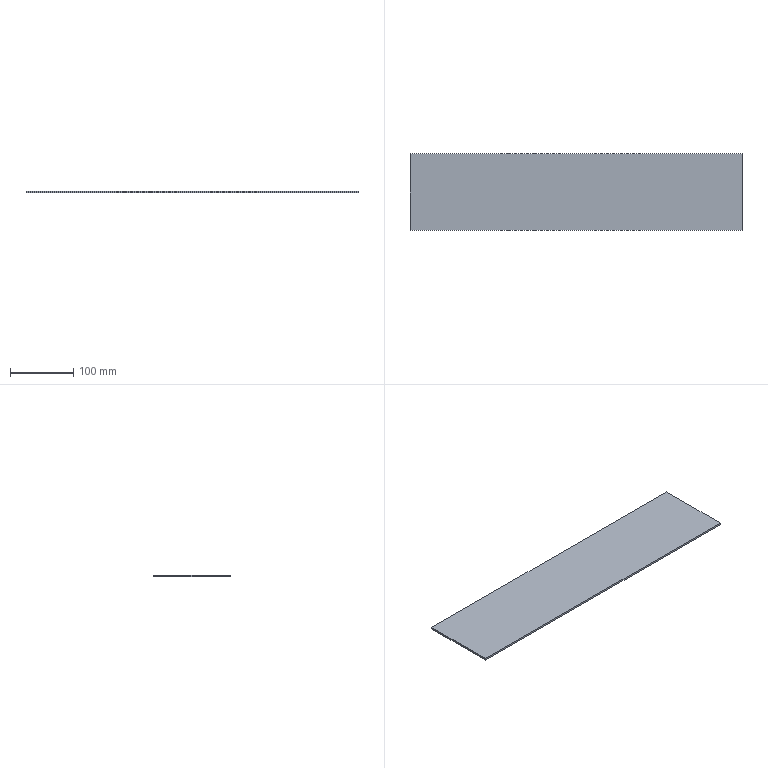Part | STEP file | Double-tube frame vertical brace plate SGN-1-06 | 1 solid | 6 faces | box 523 x 120 x 3 mm | volume 188280 mm3 | plane 6
STEP:
#1=CARTESIAN_POINT('',(0.,0.,0.));
#2=DIRECTION('',(0.,0.,1.));
#3=DIRECTION('',(1.,0.,0.));
#4=AXIS2_PLACEMENT_3D('',#1,#2,#3);
#5=CARTESIAN_POINT('',(261.5,-60.,0.));
#6=VERTEX_POINT('',#5);
#7=CARTESIAN_POINT('',(261.5,60.,0.));
#8=VERTEX_POINT('',#7);
#9=CARTESIAN_POINT('',(261.5,-60.,0.));
#10=DIRECTION('',(0.,1.,0.));
#11=VECTOR('',#10,1.);
#12=LINE('',#9,#11);
#13=CARTESIAN_POINT('',(261.5,-60.,-3.));
#14=DIRECTION('',(1.,0.,0.));
#15=DIRECTION('',(0.,0.,-1.));
#16=AXIS2_PLACEMENT_3D('',#13,#14,#15);
#17=PLANE('',#16);
#18=CARTESIAN_POINT('',(-3.,0.));
#19=DIRECTION('',(0.,1.));
#20=VECTOR('',#19,1.);
#21=LINE('',#18,#20);
#22=(GEOMETRIC_REPRESENTATION_CONTEXT(2)PARAMETRIC_REPRESENTATION_CONTEXT()REPRESENTATION_CONTEXT('',''));
#23=DEFINITIONAL_REPRESENTATION('',(#21),#22);
#24=PCURVE('',#17,#23);
#25=CARTESIAN_POINT('',(0.,0.,0.));
#26=DIRECTION('',(0.,0.,-1.));
#27=DIRECTION('',(-1.,0.,0.));
#28=AXIS2_PLACEMENT_3D('',#25,#26,#27);
#29=PLANE('',#28);
#30=CARTESIAN_POINT('',(-261.5,-60.));
#31=DIRECTION('',(0.,1.));
#32=VECTOR('',#31,1.);
#33=LINE('',#30,#32);
#34=(GEOMETRIC_REPRESENTATION_CONTEXT(2)PARAMETRIC_REPRESENTATION_CONTEXT()REPRESENTATION_CONTEXT('',''));
#35=DEFINITIONAL_REPRESENTATION('',(#33),#34);
#36=PCURVE('',#29,#35);
#37=SURFACE_CURVE('',#12,(#24,#36),.PCURVE_S1.);
#38=EDGE_CURVE('',#6,#8,#37,.T.);
#39=ORIENTED_EDGE('',*,*,#38,.F.);
#40=CARTESIAN_POINT('',(261.5,-60.,-3.));
#41=VERTEX_POINT('',#40);
#42=CARTESIAN_POINT('',(261.5,-60.,-3.));
#43=DIRECTION('',(0.,0.,1.));
#44=VECTOR('',#43,1.);
#45=LINE('',#42,#44);
#46=CARTESIAN_POINT('',(0.,0.));
#47=DIRECTION('',(-1.,0.));
#48=VECTOR('',#47,1.);
#49=LINE('',#46,#48);
#50=(GEOMETRIC_REPRESENTATION_CONTEXT(2)PARAMETRIC_REPRESENTATION_CONTEXT()REPRESENTATION_CONTEXT('',''));
#51=DEFINITIONAL_REPRESENTATION('',(#49),#50);
#52=PCURVE('',#17,#51);
#53=CARTESIAN_POINT('',(-261.5,-60.,-3.));
#54=DIRECTION('',(0.,-1.,0.));
#55=DIRECTION('',(0.,0.,-1.));
#56=AXIS2_PLACEMENT_3D('',#53,#54,#55);
#57=PLANE('',#56);
#58=CARTESIAN_POINT('',(0.,523.));
#59=DIRECTION('',(-1.,0.));
#60=VECTOR('',#59,1.);
#61=LINE('',#58,#60);
#62=(GEOMETRIC_REPRESENTATION_CONTEXT(2)PARAMETRIC_REPRESENTATION_CONTEXT()REPRESENTATION_CONTEXT('',''));
#63=DEFINITIONAL_REPRESENTATION('',(#61),#62);
#64=PCURVE('',#57,#63);
#65=SURFACE_CURVE('',#45,(#52,#64),.PCURVE_S1.);
#66=EDGE_CURVE('',#41,#6,#65,.T.);
#67=ORIENTED_EDGE('',*,*,#66,.F.);
#68=CARTESIAN_POINT('',(261.5,60.,-3.));
#69=VERTEX_POINT('',#68);
#70=CARTESIAN_POINT('',(261.5,-60.,-3.));
#71=DIRECTION('',(0.,1.,0.));
#72=VECTOR('',#71,1.);
#73=LINE('',#70,#72);
#74=CARTESIAN_POINT('',(0.,0.));
#75=DIRECTION('',(0.,1.));
#76=VECTOR('',#75,1.);
#77=LINE('',#74,#76);
#78=(GEOMETRIC_REPRESENTATION_CONTEXT(2)PARAMETRIC_REPRESENTATION_CONTEXT()REPRESENTATION_CONTEXT('',''));
#79=DEFINITIONAL_REPRESENTATION('',(#77),#78);
#80=PCURVE('',#17,#79);
#81=CARTESIAN_POINT('',(0.,0.,-3.));
#82=DIRECTION('',(0.,0.,-1.));
#83=DIRECTION('',(-1.,0.,0.));
#84=AXIS2_PLACEMENT_3D('',#81,#82,#83);
#85=PLANE('',#84);
#86=CARTESIAN_POINT('',(-261.5,-60.));
#87=DIRECTION('',(0.,1.));
#88=VECTOR('',#87,1.);
#89=LINE('',#86,#88);
#90=(GEOMETRIC_REPRESENTATION_CONTEXT(2)PARAMETRIC_REPRESENTATION_CONTEXT()REPRESENTATION_CONTEXT('',''));
#91=DEFINITIONAL_REPRESENTATION('',(#89),#90);
#92=PCURVE('',#85,#91);
#93=SURFACE_CURVE('',#73,(#80,#92),.PCURVE_S1.);
#94=EDGE_CURVE('',#41,#69,#93,.T.);
#95=ORIENTED_EDGE('',*,*,#94,.T.);
#96=CARTESIAN_POINT('',(261.5,60.,-3.));
#97=DIRECTION('',(0.,0.,1.));
#98=VECTOR('',#97,1.);
#99=LINE('',#96,#98);
#100=CARTESIAN_POINT('',(0.,120.));
#101=DIRECTION('',(-1.,0.));
#102=VECTOR('',#101,1.);
#103=LINE('',#100,#102);
#104=(GEOMETRIC_REPRESENTATION_CONTEXT(2)PARAMETRIC_REPRESENTATION_CONTEXT()REPRESENTATION_CONTEXT('',''));
#105=DEFINITIONAL_REPRESENTATION('',(#103),#104);
#106=PCURVE('',#17,#105);
#107=CARTESIAN_POINT('',(-261.5,60.,-3.));
#108=DIRECTION('',(0.,1.,0.));
#109=DIRECTION('',(0.,0.,1.));
#110=AXIS2_PLACEMENT_3D('',#107,#108,#109);
#111=PLANE('',#110);
#112=CARTESIAN_POINT('',(0.,523.));
#113=DIRECTION('',(1.,0.));
#114=VECTOR('',#113,1.);
#115=LINE('',#112,#114);
#116=(GEOMETRIC_REPRESENTATION_CONTEXT(2)PARAMETRIC_REPRESENTATION_CONTEXT()REPRESENTATION_CONTEXT('',''));
#117=DEFINITIONAL_REPRESENTATION('',(#115),#116);
#118=PCURVE('',#111,#117);
#119=SURFACE_CURVE('',#99,(#106,#118),.PCURVE_S1.);
#120=EDGE_CURVE('',#69,#8,#119,.T.);
#121=ORIENTED_EDGE('',*,*,#120,.T.);
#122=EDGE_LOOP('',(#39,#67,#95,#121));
#123=FACE_BOUND('',#122,.T.);
#124=ADVANCED_FACE('',(#123),#17,.T.);
#125=CARTESIAN_POINT('',(-261.5,-60.,0.));
#126=VERTEX_POINT('',#125);
#127=CARTESIAN_POINT('',(-261.5,-60.,0.));
#128=DIRECTION('',(1.,0.,0.));
#129=VECTOR('',#128,1.);
#130=LINE('',#127,#129);
#131=CARTESIAN_POINT('',(-3.,0.));
#132=DIRECTION('',(0.,1.));
#133=VECTOR('',#132,1.);
#134=LINE('',#131,#133);
#135=(GEOMETRIC_REPRESENTATION_CONTEXT(2)PARAMETRIC_REPRESENTATION_CONTEXT()REPRESENTATION_CONTEXT('',''));
#136=DEFINITIONAL_REPRESENTATION('',(#134),#135);
#137=PCURVE('',#57,#136);
#138=CARTESIAN_POINT('',(261.5,-60.));
#139=DIRECTION('',(-1.,0.));
#140=VECTOR('',#139,1.);
#141=LINE('',#138,#140);
#142=(GEOMETRIC_REPRESENTATION_CONTEXT(2)PARAMETRIC_REPRESENTATION_CONTEXT()REPRESENTATION_CONTEXT('',''));
#143=DEFINITIONAL_REPRESENTATION('',(#141),#142);
#144=PCURVE('',#29,#143);
#145=SURFACE_CURVE('',#130,(#137,#144),.PCURVE_S1.);
#146=EDGE_CURVE('',#126,#6,#145,.T.);
#147=ORIENTED_EDGE('',*,*,#146,.F.);
#148=CARTESIAN_POINT('',(-261.5,-60.,-3.));
#149=VERTEX_POINT('',#148);
#150=CARTESIAN_POINT('',(-261.5,-60.,-3.));
#151=DIRECTION('',(0.,0.,1.));
#152=VECTOR('',#151,1.);
#153=LINE('',#150,#152);
#154=CARTESIAN_POINT('',(0.,0.));
#155=DIRECTION('',(-1.,0.));
#156=VECTOR('',#155,1.);
#157=LINE('',#154,#156);
#158=(GEOMETRIC_REPRESENTATION_CONTEXT(2)PARAMETRIC_REPRESENTATION_CONTEXT()REPRESENTATION_CONTEXT('',''));
#159=DEFINITIONAL_REPRESENTATION('',(#157),#158);
#160=PCURVE('',#57,#159);
#161=CARTESIAN_POINT('',(-261.5,-60.,-3.));
#162=DIRECTION('',(-1.,0.,0.));
#163=DIRECTION('',(0.,0.,1.));
#164=AXIS2_PLACEMENT_3D('',#161,#162,#163);
#165=PLANE('',#164);
#166=CARTESIAN_POINT('',(0.,0.));
#167=DIRECTION('',(1.,0.));
#168=VECTOR('',#167,1.);
#169=LINE('',#166,#168);
#170=(GEOMETRIC_REPRESENTATION_CONTEXT(2)PARAMETRIC_REPRESENTATION_CONTEXT()REPRESENTATION_CONTEXT('',''));
#171=DEFINITIONAL_REPRESENTATION('',(#169),#170);
#172=PCURVE('',#165,#171);
#173=SURFACE_CURVE('',#153,(#160,#172),.PCURVE_S1.);
#174=EDGE_CURVE('',#149,#126,#173,.T.);
#175=ORIENTED_EDGE('',*,*,#174,.F.);
#176=CARTESIAN_POINT('',(-261.5,-60.,-3.));
#177=DIRECTION('',(1.,0.,0.));
#178=VECTOR('',#177,1.);
#179=LINE('',#176,#178);
#180=CARTESIAN_POINT('',(0.,0.));
#181=DIRECTION('',(0.,1.));
#182=VECTOR('',#181,1.);
#183=LINE('',#180,#182);
#184=(GEOMETRIC_REPRESENTATION_CONTEXT(2)PARAMETRIC_REPRESENTATION_CONTEXT()REPRESENTATION_CONTEXT('',''));
#185=DEFINITIONAL_REPRESENTATION('',(#183),#184);
#186=PCURVE('',#57,#185);
#187=CARTESIAN_POINT('',(261.5,-60.));
#188=DIRECTION('',(-1.,0.));
#189=VECTOR('',#188,1.);
#190=LINE('',#187,#189);
#191=(GEOMETRIC_REPRESENTATION_CONTEXT(2)PARAMETRIC_REPRESENTATION_CONTEXT()REPRESENTATION_CONTEXT('',''));
#192=DEFINITIONAL_REPRESENTATION('',(#190),#191);
#193=PCURVE('',#85,#192);
#194=SURFACE_CURVE('',#179,(#186,#193),.PCURVE_S1.);
#195=EDGE_CURVE('',#149,#41,#194,.T.);
#196=ORIENTED_EDGE('',*,*,#195,.T.);
#197=ORIENTED_EDGE('',*,*,#66,.T.);
#198=EDGE_LOOP('',(#147,#175,#196,#197));
#199=FACE_BOUND('',#198,.T.);
#200=ADVANCED_FACE('',(#199),#57,.T.);
#201=CARTESIAN_POINT('',(-261.5,60.,0.));
#202=VERTEX_POINT('',#201);
#203=CARTESIAN_POINT('',(-261.5,-60.,0.));
#204=DIRECTION('',(0.,-1.,0.));
#205=VECTOR('',#204,1.);
#206=LINE('',#203,#205);
#207=CARTESIAN_POINT('',(3.,0.));
#208=DIRECTION('',(0.,-1.));
#209=VECTOR('',#208,1.);
#210=LINE('',#207,#209);
#211=(GEOMETRIC_REPRESENTATION_CONTEXT(2)PARAMETRIC_REPRESENTATION_CONTEXT()REPRESENTATION_CONTEXT('',''));
#212=DEFINITIONAL_REPRESENTATION('',(#210),#211);
#213=PCURVE('',#165,#212);
#214=CARTESIAN_POINT('',(261.5,-60.));
#215=DIRECTION('',(0.,-1.));
#216=VECTOR('',#215,1.);
#217=LINE('',#214,#216);
#218=(GEOMETRIC_REPRESENTATION_CONTEXT(2)PARAMETRIC_REPRESENTATION_CONTEXT()REPRESENTATION_CONTEXT('',''));
#219=DEFINITIONAL_REPRESENTATION('',(#217),#218);
#220=PCURVE('',#29,#219);
#221=SURFACE_CURVE('',#206,(#213,#220),.PCURVE_S1.);
#222=EDGE_CURVE('',#202,#126,#221,.T.);
#223=ORIENTED_EDGE('',*,*,#222,.F.);
#224=CARTESIAN_POINT('',(-261.5,60.,-3.));
#225=VERTEX_POINT('',#224);
#226=CARTESIAN_POINT('',(-261.5,60.,-3.));
#227=DIRECTION('',(0.,0.,1.));
#228=VECTOR('',#227,1.);
#229=LINE('',#226,#228);
#230=CARTESIAN_POINT('',(0.,120.));
#231=DIRECTION('',(1.,0.));
#232=VECTOR('',#231,1.);
#233=LINE('',#230,#232);
#234=(GEOMETRIC_REPRESENTATION_CONTEXT(2)PARAMETRIC_REPRESENTATION_CONTEXT()REPRESENTATION_CONTEXT('',''));
#235=DEFINITIONAL_REPRESENTATION('',(#233),#234);
#236=PCURVE('',#165,#235);
#237=CARTESIAN_POINT('',(0.,0.));
#238=DIRECTION('',(1.,0.));
#239=VECTOR('',#238,1.);
#240=LINE('',#237,#239);
#241=(GEOMETRIC_REPRESENTATION_CONTEXT(2)PARAMETRIC_REPRESENTATION_CONTEXT()REPRESENTATION_CONTEXT('',''));
#242=DEFINITIONAL_REPRESENTATION('',(#240),#241);
#243=PCURVE('',#111,#242);
#244=SURFACE_CURVE('',#229,(#236,#243),.PCURVE_S1.);
#245=EDGE_CURVE('',#225,#202,#244,.T.);
#246=ORIENTED_EDGE('',*,*,#245,.F.);
#247=CARTESIAN_POINT('',(-261.5,-60.,-3.));
#248=DIRECTION('',(0.,-1.,0.));
#249=VECTOR('',#248,1.);
#250=LINE('',#247,#249);
#251=CARTESIAN_POINT('',(0.,0.));
#252=DIRECTION('',(0.,-1.));
#253=VECTOR('',#252,1.);
#254=LINE('',#251,#253);
#255=(GEOMETRIC_REPRESENTATION_CONTEXT(2)PARAMETRIC_REPRESENTATION_CONTEXT()REPRESENTATION_CONTEXT('',''));
#256=DEFINITIONAL_REPRESENTATION('',(#254),#255);
#257=PCURVE('',#165,#256);
#258=CARTESIAN_POINT('',(261.5,-60.));
#259=DIRECTION('',(0.,-1.));
#260=VECTOR('',#259,1.);
#261=LINE('',#258,#260);
#262=(GEOMETRIC_REPRESENTATION_CONTEXT(2)PARAMETRIC_REPRESENTATION_CONTEXT()REPRESENTATION_CONTEXT('',''));
#263=DEFINITIONAL_REPRESENTATION('',(#261),#262);
#264=PCURVE('',#85,#263);
#265=SURFACE_CURVE('',#250,(#257,#264),.PCURVE_S1.);
#266=EDGE_CURVE('',#225,#149,#265,.T.);
#267=ORIENTED_EDGE('',*,*,#266,.T.);
#268=ORIENTED_EDGE('',*,*,#174,.T.);
#269=EDGE_LOOP('',(#223,#246,#267,#268));
#270=FACE_BOUND('',#269,.T.);
#271=ADVANCED_FACE('',(#270),#165,.T.);
#272=CARTESIAN_POINT('',(-261.5,60.,0.));
#273=DIRECTION('',(-1.,0.,0.));
#274=VECTOR('',#273,1.);
#275=LINE('',#272,#274);
#276=CARTESIAN_POINT('',(3.,0.));
#277=DIRECTION('',(0.,-1.));
#278=VECTOR('',#277,1.);
#279=LINE('',#276,#278);
#280=(GEOMETRIC_REPRESENTATION_CONTEXT(2)PARAMETRIC_REPRESENTATION_CONTEXT()REPRESENTATION_CONTEXT('',''));
#281=DEFINITIONAL_REPRESENTATION('',(#279),#280);
#282=PCURVE('',#111,#281);
#283=CARTESIAN_POINT('',(261.5,60.));
#284=DIRECTION('',(1.,0.));
#285=VECTOR('',#284,1.);
#286=LINE('',#283,#285);
#287=(GEOMETRIC_REPRESENTATION_CONTEXT(2)PARAMETRIC_REPRESENTATION_CONTEXT()REPRESENTATION_CONTEXT('',''));
#288=DEFINITIONAL_REPRESENTATION('',(#286),#287);
#289=PCURVE('',#29,#288);
#290=SURFACE_CURVE('',#275,(#282,#289),.PCURVE_S1.);
#291=EDGE_CURVE('',#8,#202,#290,.T.);
#292=ORIENTED_EDGE('',*,*,#291,.F.);
#293=ORIENTED_EDGE('',*,*,#120,.F.);
#294=CARTESIAN_POINT('',(-261.5,60.,-3.));
#295=DIRECTION('',(-1.,0.,0.));
#296=VECTOR('',#295,1.);
#297=LINE('',#294,#296);
#298=CARTESIAN_POINT('',(0.,0.));
#299=DIRECTION('',(0.,-1.));
#300=VECTOR('',#299,1.);
#301=LINE('',#298,#300);
#302=(GEOMETRIC_REPRESENTATION_CONTEXT(2)PARAMETRIC_REPRESENTATION_CONTEXT()REPRESENTATION_CONTEXT('',''));
#303=DEFINITIONAL_REPRESENTATION('',(#301),#302);
#304=PCURVE('',#111,#303);
#305=CARTESIAN_POINT('',(261.5,60.));
#306=DIRECTION('',(1.,0.));
#307=VECTOR('',#306,1.);
#308=LINE('',#305,#307);
#309=(GEOMETRIC_REPRESENTATION_CONTEXT(2)PARAMETRIC_REPRESENTATION_CONTEXT()REPRESENTATION_CONTEXT('',''));
#310=DEFINITIONAL_REPRESENTATION('',(#308),#309);
#311=PCURVE('',#85,#310);
#312=SURFACE_CURVE('',#297,(#304,#311),.PCURVE_S1.);
#313=EDGE_CURVE('',#69,#225,#312,.T.);
#314=ORIENTED_EDGE('',*,*,#313,.T.);
#315=ORIENTED_EDGE('',*,*,#245,.T.);
#316=EDGE_LOOP('',(#292,#293,#314,#315));
#317=FACE_BOUND('',#316,.T.);
#318=ADVANCED_FACE('',(#317),#111,.T.);
#319=ORIENTED_EDGE('',*,*,#94,.F.);
#320=ORIENTED_EDGE('',*,*,#195,.F.);
#321=ORIENTED_EDGE('',*,*,#266,.F.);
#322=ORIENTED_EDGE('',*,*,#313,.F.);
#323=EDGE_LOOP('',(#319,#320,#321,#322));
#324=FACE_BOUND('',#323,.T.);
#325=ADVANCED_FACE('',(#324),#85,.T.);
#326=ORIENTED_EDGE('',*,*,#38,.T.);
#327=ORIENTED_EDGE('',*,*,#291,.T.);
#328=ORIENTED_EDGE('',*,*,#222,.T.);
#329=ORIENTED_EDGE('',*,*,#146,.T.);
#330=EDGE_LOOP('',(#326,#327,#328,#329));
#331=FACE_BOUND('',#330,.T.);
#332=ADVANCED_FACE('',(#331),#29,.F.);
#333=CLOSED_SHELL('',(#124,#200,#271,#318,#325,#332));
#334=MANIFOLD_SOLID_BREP('',#333);
#335=(LENGTH_UNIT()NAMED_UNIT(*)SI_UNIT(.MILLI.,.METRE.));
#336=UNCERTAINTY_MEASURE_WITH_UNIT(LENGTH_MEASURE(0.0000001),#335,'','');
#337=(NAMED_UNIT(*)PLANE_ANGLE_UNIT()SI_UNIT($,.RADIAN.));
#338=(NAMED_UNIT(*)SI_UNIT($,.STERADIAN.)SOLID_ANGLE_UNIT());
#339=(GEOMETRIC_REPRESENTATION_CONTEXT(3)GLOBAL_UNCERTAINTY_ASSIGNED_CONTEXT((#336))GLOBAL_UNIT_ASSIGNED_CONTEXT((#335,#337,#338))REPRESENTATION_CONTEXT('',''));
#340=ADVANCED_BREP_SHAPE_REPRESENTATION('',(#4,#334),#339);